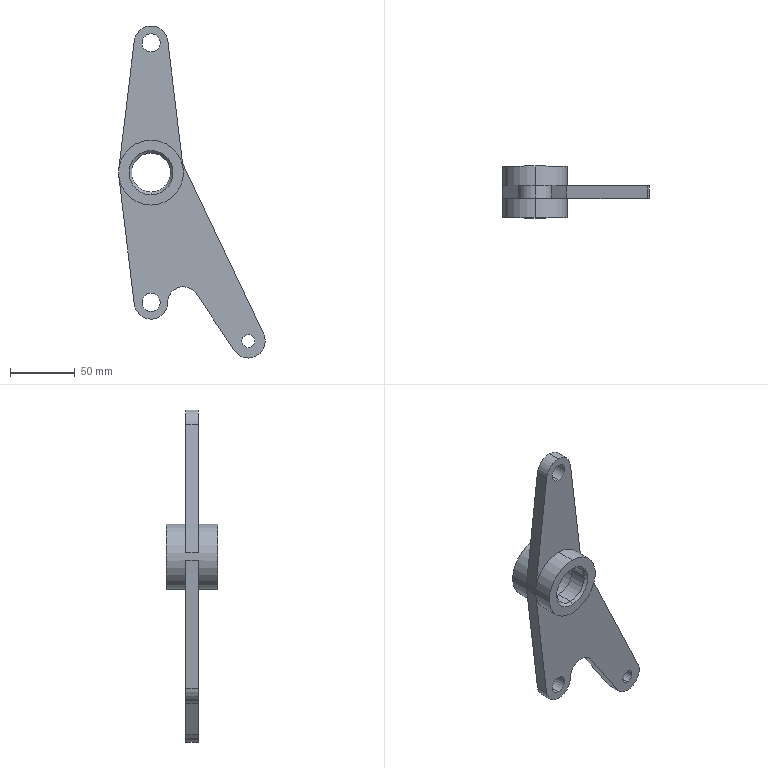Part | SolidWorks | features MirrorStock 1 | 1 solid | 37 faces | box 113 x 40 x 255.904 mm | volume 148805 mm3 | cylinder 21 | plane 12 | cone 4 | commonest cylinder face diameters 14 x4 26 x4 30 x4 50 x3 10 x2 24 x2
STEP:
#1=CARTESIAN_POINT('',(0.,-5.,-17.));
#2=VERTEX_POINT('',#1);
#3=CARTESIAN_POINT('',(0.,-5.,17.));
#4=VERTEX_POINT('',#3);
#5=CARTESIAN_POINT('',(0.,-5.,0.));
#6=DIRECTION('',(0.,-1.,0.));
#7=DIRECTION('',(0.,0.,-1.));
#8=AXIS2_PLACEMENT_3D('',#5,#6,#7);
#9=CIRCLE('',#8,17.);
#10=EDGE_CURVE('',#2,#4,#9,.T.);
#11=ORIENTED_EDGE('',*,*,#10,.T.);
#12=CARTESIAN_POINT('',(0.,5.,17.));
#13=VERTEX_POINT('',#12);
#14=CARTESIAN_POINT('',(0.,-5.,17.));
#15=DIRECTION('',(0.,1.,0.));
#16=VECTOR('',#15,1000.);
#17=LINE('',#14,#16);
#18=EDGE_CURVE('',#4,#13,#17,.T.);
#19=ORIENTED_EDGE('',*,*,#18,.T.);
#20=CARTESIAN_POINT('',(0.,5.,-17.));
#21=VERTEX_POINT('',#20);
#22=CARTESIAN_POINT('',(0.,5.,0.));
#23=DIRECTION('',(0.,-1.,0.));
#24=DIRECTION('',(0.,0.,-1.));
#25=AXIS2_PLACEMENT_3D('',#22,#23,#24);
#26=CIRCLE('',#25,17.);
#27=EDGE_CURVE('',#21,#13,#26,.T.);
#28=ORIENTED_EDGE('',*,*,#27,.F.);
#29=CARTESIAN_POINT('',(0.,-5.,-17.));
#30=DIRECTION('',(0.,1.,0.));
#31=VECTOR('',#30,1000.);
#32=LINE('',#29,#31);
#33=EDGE_CURVE('',#2,#21,#32,.T.);
#34=ORIENTED_EDGE('',*,*,#33,.F.);
#35=EDGE_LOOP('',(#11,#19,#28,#34));
#36=FACE_OUTER_BOUND('',#35,.T.);
#37=CARTESIAN_POINT('',(0.,-5.,0.));
#38=DIRECTION('',(0.,1.,0.));
#39=DIRECTION('',(0.,0.,-1.));
#40=AXIS2_PLACEMENT_3D('',#37,#38,#39);
#41=CYLINDRICAL_SURFACE('',#40,17.);
#42=ADVANCED_FACE('',(#36),#41,.F.);
#43=CARTESIAN_POINT('',(0.,18.,-15.));
#44=VERTEX_POINT('',#43);
#45=CARTESIAN_POINT('',(0.,18.,15.));
#46=VERTEX_POINT('',#45);
#47=CARTESIAN_POINT('',(0.,18.,0.));
#48=DIRECTION('',(0.,-1.,0.));
#49=DIRECTION('',(0.,0.,-1.));
#50=AXIS2_PLACEMENT_3D('',#47,#48,#49);
#51=CIRCLE('',#50,15.);
#52=EDGE_CURVE('',#44,#46,#51,.T.);
#53=ORIENTED_EDGE('',*,*,#52,.T.);
#54=CARTESIAN_POINT('',(0.,20.,17.));
#55=VERTEX_POINT('',#54);
#56=CARTESIAN_POINT('',(0.,18.,15.));
#57=DIRECTION('',(0.,0.7071,0.7071));
#58=VECTOR('',#57,1000.);
#59=LINE('',#56,#58);
#60=EDGE_CURVE('',#46,#55,#59,.T.);
#61=ORIENTED_EDGE('',*,*,#60,.T.);
#62=CARTESIAN_POINT('',(0.,20.,-17.));
#63=VERTEX_POINT('',#62);
#64=CARTESIAN_POINT('',(0.,20.,0.));
#65=DIRECTION('',(0.,1.,0.));
#66=DIRECTION('',(0.,0.,-1.));
#67=AXIS2_PLACEMENT_3D('',#64,#65,#66);
#68=CIRCLE('',#67,17.);
#69=EDGE_CURVE('',#55,#63,#68,.T.);
#70=ORIENTED_EDGE('',*,*,#69,.T.);
#71=CARTESIAN_POINT('',(0.,18.,-15.));
#72=DIRECTION('',(0.,0.7071,-0.7071));
#73=VECTOR('',#72,1000.);
#74=LINE('',#71,#73);
#75=EDGE_CURVE('',#44,#63,#74,.T.);
#76=ORIENTED_EDGE('',*,*,#75,.F.);
#77=EDGE_LOOP('',(#53,#61,#70,#76));
#78=FACE_OUTER_BOUND('',#77,.T.);
#79=CARTESIAN_POINT('',(0.,18.,0.));
#80=DIRECTION('',(0.,1.,0.));
#81=DIRECTION('',(0.,0.,-1.));
#82=AXIS2_PLACEMENT_3D('',#79,#80,#81);
#83=CONICAL_SURFACE('',#82,15.,0.7854);
#84=ADVANCED_FACE('',(#78),#83,.F.);
#85=CARTESIAN_POINT('',(0.,-18.,15.));
#86=VERTEX_POINT('',#85);
#87=CARTESIAN_POINT('',(0.,-18.,-15.));
#88=VERTEX_POINT('',#87);
#89=CARTESIAN_POINT('',(0.,-18.,0.));
#90=DIRECTION('',(0.,1.,0.));
#91=DIRECTION('',(0.,0.,-1.));
#92=AXIS2_PLACEMENT_3D('',#89,#90,#91);
#93=CIRCLE('',#92,15.);
#94=EDGE_CURVE('',#86,#88,#93,.T.);
#95=ORIENTED_EDGE('',*,*,#94,.T.);
#96=CARTESIAN_POINT('',(0.,-20.,-17.));
#97=VERTEX_POINT('',#96);
#98=CARTESIAN_POINT('',(0.,-20.,-17.));
#99=DIRECTION('',(0.,-0.7071,-0.7071));
#100=VECTOR('',#99,1000.);
#101=LINE('',#98,#100);
#102=EDGE_CURVE('',#88,#97,#101,.T.);
#103=ORIENTED_EDGE('',*,*,#102,.T.);
#104=CARTESIAN_POINT('',(0.,-20.,17.));
#105=VERTEX_POINT('',#104);
#106=CARTESIAN_POINT('',(0.,-20.,0.));
#107=DIRECTION('',(0.,-1.,0.));
#108=DIRECTION('',(0.,0.,-1.));
#109=AXIS2_PLACEMENT_3D('',#106,#107,#108);
#110=CIRCLE('',#109,17.);
#111=EDGE_CURVE('',#97,#105,#110,.T.);
#112=ORIENTED_EDGE('',*,*,#111,.T.);
#113=CARTESIAN_POINT('',(0.,-20.,17.));
#114=DIRECTION('',(0.,-0.7071,0.7071));
#115=VECTOR('',#114,1000.);
#116=LINE('',#113,#115);
#117=EDGE_CURVE('',#86,#105,#116,.T.);
#118=ORIENTED_EDGE('',*,*,#117,.F.);
#119=EDGE_LOOP('',(#95,#103,#112,#118));
#120=FACE_OUTER_BOUND('',#119,.T.);
#121=CARTESIAN_POINT('',(0.,-20.,0.));
#122=DIRECTION('',(0.,-1.,0.));
#123=DIRECTION('',(0.,0.,1.));
#124=AXIS2_PLACEMENT_3D('',#121,#122,#123);
#125=CONICAL_SURFACE('',#124,17.,0.7854);
#126=ADVANCED_FACE('',(#120),#125,.F.);
#127=CARTESIAN_POINT('',(75.,5.,-134.904));
#128=VERTEX_POINT('',#127);
#129=CARTESIAN_POINT('',(75.,5.,-124.904));
#130=VERTEX_POINT('',#129);
#131=CARTESIAN_POINT('',(75.,5.,-129.904));
#132=DIRECTION('',(0.,-1.,0.));
#133=DIRECTION('',(0.,0.,-1.));
#134=AXIS2_PLACEMENT_3D('',#131,#132,#133);
#135=CIRCLE('',#134,5.);
#136=EDGE_CURVE('',#128,#130,#135,.T.);
#137=ORIENTED_EDGE('',*,*,#136,.F.);
#138=CARTESIAN_POINT('',(75.,-5.,-134.904));
#139=VERTEX_POINT('',#138);
#140=CARTESIAN_POINT('',(75.,5.,-134.904));
#141=DIRECTION('',(0.,-1.,0.));
#142=VECTOR('',#141,1000.);
#143=LINE('',#140,#142);
#144=EDGE_CURVE('',#128,#139,#143,.T.);
#145=ORIENTED_EDGE('',*,*,#144,.T.);
#146=CARTESIAN_POINT('',(75.,-5.,-124.904));
#147=VERTEX_POINT('',#146);
#148=CARTESIAN_POINT('',(75.,-5.,-129.904));
#149=DIRECTION('',(0.,-1.,0.));
#150=DIRECTION('',(0.,0.,-1.));
#151=AXIS2_PLACEMENT_3D('',#148,#149,#150);
#152=CIRCLE('',#151,5.);
#153=EDGE_CURVE('',#139,#147,#152,.T.);
#154=ORIENTED_EDGE('',*,*,#153,.T.);
#155=CARTESIAN_POINT('',(75.,5.,-124.904));
#156=DIRECTION('',(0.,-1.,0.));
#157=VECTOR('',#156,1000.);
#158=LINE('',#155,#157);
#159=EDGE_CURVE('',#130,#147,#158,.T.);
#160=ORIENTED_EDGE('',*,*,#159,.F.);
#161=EDGE_LOOP('',(#137,#145,#154,#160));
#162=FACE_OUTER_BOUND('',#161,.T.);
#163=CARTESIAN_POINT('',(75.,5.,-129.904));
#164=DIRECTION('',(0.,-1.,0.));
#165=DIRECTION('',(0.,0.,1.));
#166=AXIS2_PLACEMENT_3D('',#163,#164,#165);
#167=CYLINDRICAL_SURFACE('',#166,5.);
#168=ADVANCED_FACE('',(#162),#167,.F.);
#169=CARTESIAN_POINT('',(0.,5.,-107.));
#170=VERTEX_POINT('',#169);
#171=CARTESIAN_POINT('',(0.,5.,-93.));
#172=VERTEX_POINT('',#171);
#173=CARTESIAN_POINT('',(0.,5.,-100.));
#174=DIRECTION('',(0.,-1.,0.));
#175=DIRECTION('',(0.,0.,1.));
#176=AXIS2_PLACEMENT_3D('',#173,#174,#175);
#177=CIRCLE('',#176,7.);
#178=EDGE_CURVE('',#170,#172,#177,.T.);
#179=ORIENTED_EDGE('',*,*,#178,.F.);
#180=CARTESIAN_POINT('',(0.,-5.,-107.));
#181=VERTEX_POINT('',#180);
#182=CARTESIAN_POINT('',(0.,5.,-107.));
#183=DIRECTION('',(0.,-1.,0.));
#184=VECTOR('',#183,1000.);
#185=LINE('',#182,#184);
#186=EDGE_CURVE('',#170,#181,#185,.T.);
#187=ORIENTED_EDGE('',*,*,#186,.T.);
#188=CARTESIAN_POINT('',(0.,-5.,-93.));
#189=VERTEX_POINT('',#188);
#190=CARTESIAN_POINT('',(0.,-5.,-100.));
#191=DIRECTION('',(0.,-1.,0.));
#192=DIRECTION('',(0.,0.,1.));
#193=AXIS2_PLACEMENT_3D('',#190,#191,#192);
#194=CIRCLE('',#193,7.);
#195=EDGE_CURVE('',#181,#189,#194,.T.);
#196=ORIENTED_EDGE('',*,*,#195,.T.);
#197=CARTESIAN_POINT('',(0.,5.,-93.));
#198=DIRECTION('',(0.,-1.,0.));
#199=VECTOR('',#198,1000.);
#200=LINE('',#197,#199);
#201=EDGE_CURVE('',#172,#189,#200,.T.);
#202=ORIENTED_EDGE('',*,*,#201,.F.);
#203=EDGE_LOOP('',(#179,#187,#196,#202));
#204=FACE_OUTER_BOUND('',#203,.T.);
#205=CARTESIAN_POINT('',(0.,5.,-100.));
#206=DIRECTION('',(0.,-1.,0.));
#207=DIRECTION('',(0.,0.,1.));
#208=AXIS2_PLACEMENT_3D('',#205,#206,#207);
#209=CYLINDRICAL_SURFACE('',#208,7.);
#210=ADVANCED_FACE('',(#204),#209,.F.);
#211=CARTESIAN_POINT('',(0.,5.,93.));
#212=VERTEX_POINT('',#211);
#213=CARTESIAN_POINT('',(0.,5.,107.));
#214=VERTEX_POINT('',#213);
#215=CARTESIAN_POINT('',(0.,5.,100.));
#216=DIRECTION('',(0.,-1.,0.));
#217=DIRECTION('',(0.,0.,-1.));
#218=AXIS2_PLACEMENT_3D('',#215,#216,#217);
#219=CIRCLE('',#218,7.);
#220=EDGE_CURVE('',#212,#214,#219,.T.);
#221=ORIENTED_EDGE('',*,*,#220,.F.);
#222=CARTESIAN_POINT('',(0.,-5.,93.));
#223=VERTEX_POINT('',#222);
#224=CARTESIAN_POINT('',(0.,5.,93.));
#225=DIRECTION('',(0.,-1.,0.));
#226=VECTOR('',#225,1000.);
#227=LINE('',#224,#226);
#228=EDGE_CURVE('',#212,#223,#227,.T.);
#229=ORIENTED_EDGE('',*,*,#228,.T.);
#230=CARTESIAN_POINT('',(0.,-5.,107.));
#231=VERTEX_POINT('',#230);
#232=CARTESIAN_POINT('',(0.,-5.,100.));
#233=DIRECTION('',(0.,-1.,0.));
#234=DIRECTION('',(0.,0.,-1.));
#235=AXIS2_PLACEMENT_3D('',#232,#233,#234);
#236=CIRCLE('',#235,7.);
#237=EDGE_CURVE('',#223,#231,#236,.T.);
#238=ORIENTED_EDGE('',*,*,#237,.T.);
#239=CARTESIAN_POINT('',(0.,5.,107.));
#240=DIRECTION('',(0.,-1.,0.));
#241=VECTOR('',#240,1000.);
#242=LINE('',#239,#241);
#243=EDGE_CURVE('',#214,#231,#242,.T.);
#244=ORIENTED_EDGE('',*,*,#243,.F.);
#245=EDGE_LOOP('',(#221,#229,#238,#244));
#246=FACE_OUTER_BOUND('',#245,.T.);
#247=CARTESIAN_POINT('',(0.,5.,100.));
#248=DIRECTION('',(0.,-1.,0.));
#249=DIRECTION('',(0.,0.,1.));
#250=AXIS2_PLACEMENT_3D('',#247,#248,#249);
#251=CYLINDRICAL_SURFACE('',#250,7.);
#252=ADVANCED_FACE('',(#246),#251,.F.);
#253=CARTESIAN_POINT('',(12.969,5.,-101.042));
#254=VERTEX_POINT('',#253);
#255=CARTESIAN_POINT('',(24.918,5.,-87.94));
#256=VERTEX_POINT('',#255);
#257=CARTESIAN_POINT('',(24.918,5.,-99.94));
#258=DIRECTION('',(0.,1.,0.));
#259=DIRECTION('',(0.,0.,-1.));
#260=AXIS2_PLACEMENT_3D('',#257,#258,#259);
#261=CIRCLE('',#260,12.);
#262=EDGE_CURVE('',#254,#256,#261,.T.);
#263=ORIENTED_EDGE('',*,*,#262,.T.);
#264=CARTESIAN_POINT('',(24.918,-5.,-87.94));
#265=VERTEX_POINT('',#264);
#266=CARTESIAN_POINT('',(24.918,5.,-87.94));
#267=DIRECTION('',(0.,-1.,0.));
#268=VECTOR('',#267,1000.);
#269=LINE('',#266,#268);
#270=EDGE_CURVE('',#256,#265,#269,.T.);
#271=ORIENTED_EDGE('',*,*,#270,.T.);
#272=CARTESIAN_POINT('',(12.969,-5.,-101.042));
#273=VERTEX_POINT('',#272);
#274=CARTESIAN_POINT('',(24.918,-5.,-99.94));
#275=DIRECTION('',(0.,1.,0.));
#276=DIRECTION('',(0.,0.,-1.));
#277=AXIS2_PLACEMENT_3D('',#274,#275,#276);
#278=CIRCLE('',#277,12.);
#279=EDGE_CURVE('',#273,#265,#278,.T.);
#280=ORIENTED_EDGE('',*,*,#279,.F.);
#281=CARTESIAN_POINT('',(12.969,5.,-101.042));
#282=DIRECTION('',(0.,-1.,0.));
#283=VECTOR('',#282,1000.);
#284=LINE('',#281,#283);
#285=EDGE_CURVE('',#254,#273,#284,.T.);
#286=ORIENTED_EDGE('',*,*,#285,.F.);
#287=EDGE_LOOP('',(#263,#271,#280,#286));
#288=FACE_OUTER_BOUND('',#287,.T.);
#289=CARTESIAN_POINT('',(24.918,5.,-99.94));
#290=DIRECTION('',(0.,-1.,0.));
#291=DIRECTION('',(0.,0.,1.));
#292=AXIS2_PLACEMENT_3D('',#289,#290,#291);
#293=CYLINDRICAL_SURFACE('',#292,12.);
#294=ADVANCED_FACE('',(#288),#293,.F.);
#295=CARTESIAN_POINT('',(12.906,5.,101.56));
#296=VERTEX_POINT('',#295);
#297=CARTESIAN_POINT('',(0.,5.,113.));
#298=VERTEX_POINT('',#297);
#299=CARTESIAN_POINT('',(0.,5.,100.));
#300=DIRECTION('',(0.,-1.,0.));
#301=DIRECTION('',(0.,0.,-1.));
#302=AXIS2_PLACEMENT_3D('',#299,#300,#301);
#303=CIRCLE('',#302,13.);
#304=EDGE_CURVE('',#296,#298,#303,.T.);
#305=ORIENTED_EDGE('',*,*,#304,.T.);
#306=CARTESIAN_POINT('',(0.,-5.,113.));
#307=VERTEX_POINT('',#306);
#308=CARTESIAN_POINT('',(0.,5.,113.));
#309=DIRECTION('',(0.,-1.,0.));
#310=VECTOR('',#309,1000.);
#311=LINE('',#308,#310);
#312=EDGE_CURVE('',#298,#307,#311,.T.);
#313=ORIENTED_EDGE('',*,*,#312,.T.);
#314=CARTESIAN_POINT('',(12.906,-5.,101.56));
#315=VERTEX_POINT('',#314);
#316=CARTESIAN_POINT('',(0.,-5.,100.));
#317=DIRECTION('',(0.,-1.,0.));
#318=DIRECTION('',(0.,0.,-1.));
#319=AXIS2_PLACEMENT_3D('',#316,#317,#318);
#320=CIRCLE('',#319,13.);
#321=EDGE_CURVE('',#315,#307,#320,.T.);
#322=ORIENTED_EDGE('',*,*,#321,.F.);
#323=CARTESIAN_POINT('',(12.906,5.,101.56));
#324=DIRECTION('',(0.,-1.,0.));
#325=VECTOR('',#324,1000.);
#326=LINE('',#323,#325);
#327=EDGE_CURVE('',#296,#315,#326,.T.);
#328=ORIENTED_EDGE('',*,*,#327,.F.);
#329=EDGE_LOOP('',(#305,#313,#322,#328));
#330=FACE_OUTER_BOUND('',#329,.T.);
#331=CARTESIAN_POINT('',(0.,5.,100.));
#332=DIRECTION('',(0.,-1.,0.));
#333=DIRECTION('',(0.,0.,1.));
#334=AXIS2_PLACEMENT_3D('',#331,#332,#333);
#335=CYLINDRICAL_SURFACE('',#334,13.);
#336=ADVANCED_FACE('',(#330),#335,.T.);
#337=ORIENTED_EDGE('',*,*,#52,.F.);
#338=CARTESIAN_POINT('',(0.,5.,-15.));
#339=VERTEX_POINT('',#338);
#340=CARTESIAN_POINT('',(0.,20.,-15.));
#341=DIRECTION('',(0.,-1.,0.));
#342=VECTOR('',#341,1000.);
#343=LINE('',#340,#342);
#344=EDGE_CURVE('',#44,#339,#343,.T.);
#345=ORIENTED_EDGE('',*,*,#344,.T.);
#346=CARTESIAN_POINT('',(0.,5.,15.));
#347=VERTEX_POINT('',#346);
#348=CARTESIAN_POINT('',(0.,5.,0.));
#349=DIRECTION('',(0.,-1.,0.));
#350=DIRECTION('',(0.,0.,-1.));
#351=AXIS2_PLACEMENT_3D('',#348,#349,#350);
#352=CIRCLE('',#351,15.);
#353=EDGE_CURVE('',#339,#347,#352,.T.);
#354=ORIENTED_EDGE('',*,*,#353,.T.);
#355=CARTESIAN_POINT('',(0.,20.,15.));
#356=DIRECTION('',(0.,-1.,0.));
#357=VECTOR('',#356,1000.);
#358=LINE('',#355,#357);
#359=EDGE_CURVE('',#46,#347,#358,.T.);
#360=ORIENTED_EDGE('',*,*,#359,.F.);
#361=EDGE_LOOP('',(#337,#345,#354,#360));
#362=FACE_OUTER_BOUND('',#361,.T.);
#363=CARTESIAN_POINT('',(0.,20.,0.));
#364=DIRECTION('',(0.,-1.,0.));
#365=DIRECTION('',(0.,0.,1.));
#366=AXIS2_PLACEMENT_3D('',#363,#364,#365);
#367=CYLINDRICAL_SURFACE('',#366,15.);
#368=ADVANCED_FACE('',(#362),#367,.F.);
#369=CARTESIAN_POINT('',(0.,20.,25.));
#370=VERTEX_POINT('',#369);
#371=CARTESIAN_POINT('',(0.,20.,-25.));
#372=VERTEX_POINT('',#371);
#373=CARTESIAN_POINT('',(0.,20.,0.));
#374=DIRECTION('',(0.,-1.,0.));
#375=DIRECTION('',(0.,0.,-1.));
#376=AXIS2_PLACEMENT_3D('',#373,#374,#375);
#377=CIRCLE('',#376,25.);
#378=EDGE_CURVE('',#370,#372,#377,.T.);
#379=ORIENTED_EDGE('',*,*,#378,.T.);
#380=CARTESIAN_POINT('',(0.,5.,-25.));
#381=VERTEX_POINT('',#380);
#382=CARTESIAN_POINT('',(0.,20.,-25.));
#383=DIRECTION('',(0.,-1.,0.));
#384=VECTOR('',#383,1000.);
#385=LINE('',#382,#384);
#386=EDGE_CURVE('',#372,#381,#385,.T.);
#387=ORIENTED_EDGE('',*,*,#386,.T.);
#388=CARTESIAN_POINT('',(-24.819,5.,-3.));
#389=VERTEX_POINT('',#388);
#390=CARTESIAN_POINT('',(0.,5.,0.));
#391=DIRECTION('',(0.,-1.,0.));
#392=DIRECTION('',(0.,0.,-1.));
#393=AXIS2_PLACEMENT_3D('',#390,#391,#392);
#394=CIRCLE('',#393,25.);
#395=EDGE_CURVE('',#389,#381,#394,.T.);
#396=ORIENTED_EDGE('',*,*,#395,.F.);
#397=CARTESIAN_POINT('',(-24.819,-5.,-3.));
#398=VERTEX_POINT('',#397);
#399=CARTESIAN_POINT('',(-24.819,5.,-3.));
#400=DIRECTION('',(0.,-1.,0.));
#401=VECTOR('',#400,1000.);
#402=LINE('',#399,#401);
#403=EDGE_CURVE('',#389,#398,#402,.T.);
#404=ORIENTED_EDGE('',*,*,#403,.T.);
#405=CARTESIAN_POINT('',(0.,-5.,-25.));
#406=VERTEX_POINT('',#405);
#407=CARTESIAN_POINT('',(0.,-5.,0.));
#408=DIRECTION('',(0.,-1.,0.));
#409=DIRECTION('',(0.,0.,-1.));
#410=AXIS2_PLACEMENT_3D('',#407,#408,#409);
#411=CIRCLE('',#410,25.);
#412=EDGE_CURVE('',#398,#406,#411,.T.);
#413=ORIENTED_EDGE('',*,*,#412,.T.);
#414=CARTESIAN_POINT('',(0.,-20.,-25.));
#415=VERTEX_POINT('',#414);
#416=CARTESIAN_POINT('',(0.,20.,-25.));
#417=DIRECTION('',(0.,-1.,0.));
#418=VECTOR('',#417,1000.);
#419=LINE('',#416,#418);
#420=EDGE_CURVE('',#406,#415,#419,.T.);
#421=ORIENTED_EDGE('',*,*,#420,.T.);
#422=CARTESIAN_POINT('',(0.,-20.,25.));
#423=VERTEX_POINT('',#422);
#424=CARTESIAN_POINT('',(0.,-20.,0.));
#425=DIRECTION('',(0.,-1.,0.));
#426=DIRECTION('',(0.,0.,-1.));
#427=AXIS2_PLACEMENT_3D('',#424,#425,#426);
#428=CIRCLE('',#427,25.);
#429=EDGE_CURVE('',#423,#415,#428,.T.);
#430=ORIENTED_EDGE('',*,*,#429,.F.);
#431=CARTESIAN_POINT('',(0.,-5.,25.));
#432=VERTEX_POINT('',#431);
#433=CARTESIAN_POINT('',(0.,20.,25.));
#434=DIRECTION('',(0.,-1.,0.));
#435=VECTOR('',#434,1000.);
#436=LINE('',#433,#435);
#437=EDGE_CURVE('',#432,#423,#436,.T.);
#438=ORIENTED_EDGE('',*,*,#437,.F.);
#439=CARTESIAN_POINT('',(-24.819,-5.,3.));
#440=VERTEX_POINT('',#439);
#441=CARTESIAN_POINT('',(0.,-5.,0.));
#442=DIRECTION('',(0.,-1.,0.));
#443=DIRECTION('',(0.,0.,-1.));
#444=AXIS2_PLACEMENT_3D('',#441,#442,#443);
#445=CIRCLE('',#444,25.);
#446=EDGE_CURVE('',#432,#440,#445,.T.);
#447=ORIENTED_EDGE('',*,*,#446,.T.);
#448=CARTESIAN_POINT('',(-24.819,5.,3.));
#449=VERTEX_POINT('',#448);
#450=CARTESIAN_POINT('',(-24.819,5.,3.));
#451=DIRECTION('',(0.,-1.,0.));
#452=VECTOR('',#451,1000.);
#453=LINE('',#450,#452);
#454=EDGE_CURVE('',#449,#440,#453,.T.);
#455=ORIENTED_EDGE('',*,*,#454,.F.);
#456=CARTESIAN_POINT('',(0.,5.,25.));
#457=VERTEX_POINT('',#456);
#458=CARTESIAN_POINT('',(0.,5.,0.));
#459=DIRECTION('',(0.,-1.,0.));
#460=DIRECTION('',(0.,0.,-1.));
#461=AXIS2_PLACEMENT_3D('',#458,#459,#460);
#462=CIRCLE('',#461,25.);
#463=EDGE_CURVE('',#457,#449,#462,.T.);
#464=ORIENTED_EDGE('',*,*,#463,.F.);
#465=CARTESIAN_POINT('',(0.,20.,25.));
#466=DIRECTION('',(0.,-1.,0.));
#467=VECTOR('',#466,1000.);
#468=LINE('',#465,#467);
#469=EDGE_CURVE('',#370,#457,#468,.T.);
#470=ORIENTED_EDGE('',*,*,#469,.F.);
#471=EDGE_LOOP('',(#379,#387,#396,#404,#413,#421,#430,#438,#447,#455,#464,#470));
#472=FACE_OUTER_BOUND('',#471,.T.);
#473=CARTESIAN_POINT('',(0.,20.,0.));
#474=DIRECTION('',(0.,-1.,0.));
#475=DIRECTION('',(0.,0.,1.));
#476=AXIS2_PLACEMENT_3D('',#473,#474,#475);
#477=CYLINDRICAL_SURFACE('',#476,25.);
#478=ADVANCED_FACE('',(#472),#477,.T.);
#479=ORIENTED_EDGE('',*,*,#386,.F.);
#480=CARTESIAN_POINT('',(0.,20.,0.));
#481=DIRECTION('',(0.,-1.,0.));
#482=DIRECTION('',(0.,0.,-1.));
#483=AXIS2_PLACEMENT_3D('',#480,#481,#482);
#484=CIRCLE('',#483,25.);
#485=EDGE_CURVE('',#372,#370,#484,.T.);
#486=ORIENTED_EDGE('',*,*,#485,.T.);
#487=ORIENTED_EDGE('',*,*,#469,.T.);
#488=CARTESIAN_POINT('',(0.,5.,0.));
#489=DIRECTION('',(0.,-1.,0.));
#490=DIRECTION('',(0.,0.,-1.));
#491=AXIS2_PLACEMENT_3D('',#488,#489,#490);
#492=CIRCLE('',#491,25.);
#493=EDGE_CURVE('',#381,#457,#492,.T.);
#494=ORIENTED_EDGE('',*,*,#493,.F.);
#495=EDGE_LOOP('',(#479,#486,#487,#494));
#496=FACE_OUTER_BOUND('',#495,.T.);
#497=CARTESIAN_POINT('',(0.,20.,0.));
#498=DIRECTION('',(0.,-1.,0.));
#499=DIRECTION('',(0.,0.,1.));
#500=AXIS2_PLACEMENT_3D('',#497,#498,#499);
#501=CYLINDRICAL_SURFACE('',#500,25.);
#502=ADVANCED_FACE('',(#496),#501,.T.);
#503=CARTESIAN_POINT('',(0.,-5.,-15.));
#504=VERTEX_POINT('',#503);
#505=CARTESIAN_POINT('',(0.,-5.,15.));
#506=VERTEX_POINT('',#505);
#507=CARTESIAN_POINT('',(0.,-5.,0.));
#508=DIRECTION('',(0.,-1.,0.));
#509=DIRECTION('',(0.,0.,-1.));
#510=AXIS2_PLACEMENT_3D('',#507,#508,#509);
#511=CIRCLE('',#510,15.);
#512=EDGE_CURVE('',#504,#506,#511,.T.);
#513=ORIENTED_EDGE('',*,*,#512,.F.);
#514=CARTESIAN_POINT('',(0.,20.,-15.));
#515=DIRECTION('',(0.,-1.,0.));
#516=VECTOR('',#515,1000.);
#517=LINE('',#514,#516);
#518=EDGE_CURVE('',#504,#88,#517,.T.);
#519=ORIENTED_EDGE('',*,*,#518,.T.);
#520=ORIENTED_EDGE('',*,*,#94,.F.);
#521=CARTESIAN_POINT('',(0.,20.,15.));
#522=DIRECTION('',(0.,-1.,0.));
#523=VECTOR('',#522,1000.);
#524=LINE('',#521,#523);
#525=EDGE_CURVE('',#506,#86,#524,.T.);
#526=ORIENTED_EDGE('',*,*,#525,.F.);
#527=EDGE_LOOP('',(#513,#519,#520,#526));
#528=FACE_OUTER_BOUND('',#527,.T.);
#529=CARTESIAN_POINT('',(0.,20.,0.));
#530=DIRECTION('',(0.,-1.,0.));
#531=DIRECTION('',(0.,0.,1.));
#532=AXIS2_PLACEMENT_3D('',#529,#530,#531);
#533=CYLINDRICAL_SURFACE('',#532,15.);
#534=ADVANCED_FACE('',(#528),#533,.F.);
#535=ORIENTED_EDGE('',*,*,#518,.F.);
#536=CARTESIAN_POINT('',(0.,-5.,0.));
#537=DIRECTION('',(0.,-1.,0.));
#538=DIRECTION('',(0.,0.,-1.));
#539=AXIS2_PLACEMENT_3D('',#536,#537,#538);
#540=CIRCLE('',#539,15.);
#541=EDGE_CURVE('',#506,#504,#540,.T.);
#542=ORIENTED_EDGE('',*,*,#541,.F.);
#543=ORIENTED_EDGE('',*,*,#525,.T.);
#544=CARTESIAN_POINT('',(0.,-18.,0.));
#545=DIRECTION('',(0.,1.,0.));
#546=DIRECTION('',(0.,0.,-1.));
#547=AXIS2_PLACEMENT_3D('',#544,#545,#546);
#548=CIRCLE('',#547,15.);
#549=EDGE_CURVE('',#88,#86,#548,.T.);
#550=ORIENTED_EDGE('',*,*,#549,.F.);
#551=EDGE_LOOP('',(#535,#542,#543,#550));
#552=FACE_OUTER_BOUND('',#551,.T.);
#553=CARTESIAN_POINT('',(0.,20.,0.));
#554=DIRECTION('',(0.,-1.,0.));
#555=DIRECTION('',(0.,0.,1.));
#556=AXIS2_PLACEMENT_3D('',#553,#554,#555);
#557=CYLINDRICAL_SURFACE('',#556,15.);
#558=ADVANCED_FACE('',(#552),#557,.F.);
#559=CARTESIAN_POINT('',(0.,20.,0.));
#560=DIRECTION('',(0.,1.,0.));
#561=DIRECTION('',(0.,0.,-1.));
#562=AXIS2_PLACEMENT_3D('',#559,#560,#561);
#563=CIRCLE('',#562,17.);
#564=EDGE_CURVE('',#63,#55,#563,.T.);
#565=ORIENTED_EDGE('',*,*,#564,.F.);
#566=ORIENTED_EDGE('',*,*,#69,.F.);
#567=EDGE_LOOP('',(#565,#566));
#568=FACE_BOUND('',#567,.T.);
#569=ORIENTED_EDGE('',*,*,#378,.F.);
#570=ORIENTED_EDGE('',*,*,#485,.F.);
#571=EDGE_LOOP('',(#569,#570));
#572=FACE_OUTER_BOUND('',#571,.T.);
#573=CARTESIAN_POINT('',(0.,20.,0.));
#574=DIRECTION('',(0.,1.,0.));
#575=DIRECTION('',(0.,0.,-1.));
#576=AXIS2_PLACEMENT_3D('',#573,#574,#575);
#577=PLANE('',#576);
#578=ADVANCED_FACE('',(#568,#572),#577,.T.);
#579=CARTESIAN_POINT('',(0.,-20.,0.));
#580=DIRECTION('',(0.,-1.,0.));
#581=DIRECTION('',(0.,0.,-1.));
#582=AXIS2_PLACEMENT_3D('',#579,#580,#581);
#583=CIRCLE('',#582,17.);
#584=EDGE_CURVE('',#105,#97,#583,.T.);
#585=ORIENTED_EDGE('',*,*,#584,.F.);
#586=ORIENTED_EDGE('',*,*,#111,.F.);
#587=EDGE_LOOP('',(#585,#586));
#588=FACE_BOUND('',#587,.T.);
#589=ORIENTED_EDGE('',*,*,#429,.T.);
#590=CARTESIAN_POINT('',(0.,-20.,0.));
#591=DIRECTION('',(0.,-1.,0.));
#592=DIRECTION('',(0.,0.,-1.));
#593=AXIS2_PLACEMENT_3D('',#590,#591,#592);
#594=CIRCLE('',#593,25.);
#595=EDGE_CURVE('',#415,#423,#594,.T.);
#596=ORIENTED_EDGE('',*,*,#595,.T.);
#597=EDGE_LOOP('',(#589,#596));
#598=FACE_OUTER_BOUND('',#597,.T.);
#599=CARTESIAN_POINT('',(0.,-20.,0.));
#600=DIRECTION('',(0.,1.,0.));
#601=DIRECTION('',(0.,0.,-1.));
#602=AXIS2_PLACEMENT_3D('',#599,#600,#601);
#603=PLANE('',#602);
#604=ADVANCED_FACE('',(#588,#598),#603,.F.);
#605=ORIENTED_EDGE('',*,*,#420,.F.);
#606=CARTESIAN_POINT('',(0.,-5.,0.));
#607=DIRECTION('',(0.,-1.,0.));
#608=DIRECTION('',(0.,0.,-1.));
#609=AXIS2_PLACEMENT_3D('',#606,#607,#608);
#610=CIRCLE('',#609,25.);
#611=EDGE_CURVE('',#406,#432,#610,.T.);
#612=ORIENTED_EDGE('',*,*,#611,.T.);
#613=ORIENTED_EDGE('',*,*,#437,.T.);
#614=ORIENTED_EDGE('',*,*,#595,.F.);
#615=EDGE_LOOP('',(#605,#612,#613,#614));
#616=FACE_OUTER_BOUND('',#615,.T.);
#617=CARTESIAN_POINT('',(0.,20.,0.));
#618=DIRECTION('',(0.,-1.,0.));
#619=DIRECTION('',(0.,0.,1.));
#620=AXIS2_PLACEMENT_3D('',#617,#618,#619);
#621=CYLINDRICAL_SURFACE('',#620,25.);
#622=ADVANCED_FACE('',(#616),#621,.T.);
#623=ORIENTED_EDGE('',*,*,#344,.F.);
#624=CARTESIAN_POINT('',(0.,18.,0.));
#625=DIRECTION('',(0.,-1.,0.));
#626=DIRECTION('',(0.,0.,-1.));
#627=AXIS2_PLACEMENT_3D('',#624,#625,#626);
#628=CIRCLE('',#627,15.);
#629=EDGE_CURVE('',#46,#44,#628,.T.);
#630=ORIENTED_EDGE('',*,*,#629,.F.);
#631=ORIENTED_EDGE('',*,*,#359,.T.);
#632=CARTESIAN_POINT('',(0.,5.,0.));
#633=DIRECTION('',(0.,-1.,0.));
#634=DIRECTION('',(0.,0.,-1.));
#635=AXIS2_PLACEMENT_3D('',#632,#633,#634);
#636=CIRCLE('',#635,15.);
#637=EDGE_CURVE('',#347,#339,#636,.T.);
#638=ORIENTED_EDGE('',*,*,#637,.T.);
#639=EDGE_LOOP('',(#623,#630,#631,#638));
#640=FACE_OUTER_BOUND('',#639,.T.);
#641=CARTESIAN_POINT('',(0.,20.,0.));
#642=DIRECTION('',(0.,-1.,0.));
#643=DIRECTION('',(0.,0.,1.));
#644=AXIS2_PLACEMENT_3D('',#641,#642,#643);
#645=CYLINDRICAL_SURFACE('',#644,15.);
#646=ADVANCED_FACE('',(#640),#645,.F.);
#647=CARTESIAN_POINT('',(75.,5.,-129.904));
#648=DIRECTION('',(0.,-1.,0.));
#649=DIRECTION('',(0.,0.,-1.));
#650=AXIS2_PLACEMENT_3D('',#647,#648,#649);
#651=CIRCLE('',#650,5.);
#652=EDGE_CURVE('',#130,#128,#651,.T.);
#653=ORIENTED_EDGE('',*,*,#652,.T.);
#654=ORIENTED_EDGE('',*,*,#136,.T.);
#655=EDGE_LOOP('',(#653,#654));
#656=FACE_BOUND('',#655,.T.);
#657=CARTESIAN_POINT('',(0.,5.,100.));
#658=DIRECTION('',(0.,-1.,0.));
#659=DIRECTION('',(0.,0.,-1.));
#660=AXIS2_PLACEMENT_3D('',#657,#658,#659);
#661=CIRCLE('',#660,7.);
#662=EDGE_CURVE('',#214,#212,#661,.T.);
#663=ORIENTED_EDGE('',*,*,#662,.T.);
#664=ORIENTED_EDGE('',*,*,#220,.T.);
#665=EDGE_LOOP('',(#663,#664));
#666=FACE_BOUND('',#665,.T.);
#667=CARTESIAN_POINT('',(0.,5.,-100.));
#668=DIRECTION('',(0.,-1.,0.));
#669=DIRECTION('',(0.,0.,1.));
#670=AXIS2_PLACEMENT_3D('',#667,#668,#669);
#671=CIRCLE('',#670,7.);
#672=EDGE_CURVE('',#172,#170,#671,.T.);
#673=ORIENTED_EDGE('',*,*,#672,.T.);
#674=ORIENTED_EDGE('',*,*,#178,.T.);
#675=EDGE_LOOP('',(#673,#674));
#676=FACE_BOUND('',#675,.T.);
#677=ORIENTED_EDGE('',*,*,#395,.T.);
#678=ORIENTED_EDGE('',*,*,#493,.T.);
#679=ORIENTED_EDGE('',*,*,#463,.T.);
#680=CARTESIAN_POINT('',(-12.906,5.,101.56));
#681=VERTEX_POINT('',#680);
#682=CARTESIAN_POINT('',(-12.906,5.,101.56));
#683=DIRECTION('',(-0.12,0.,-0.9928));
#684=VECTOR('',#683,1000.);
#685=LINE('',#682,#684);
#686=EDGE_CURVE('',#681,#449,#685,.T.);
#687=ORIENTED_EDGE('',*,*,#686,.F.);
#688=CARTESIAN_POINT('',(0.,5.,100.));
#689=DIRECTION('',(0.,-1.,0.));
#690=DIRECTION('',(0.,0.,-1.));
#691=AXIS2_PLACEMENT_3D('',#688,#689,#690);
#692=CIRCLE('',#691,13.);
#693=EDGE_CURVE('',#298,#681,#692,.T.);
#694=ORIENTED_EDGE('',*,*,#693,.F.);
#695=ORIENTED_EDGE('',*,*,#304,.F.);
#696=CARTESIAN_POINT('',(24.33,5.,7.046));
#697=VERTEX_POINT('',#696);
#698=CARTESIAN_POINT('',(12.906,5.,101.56));
#699=DIRECTION('',(-0.12,0.,0.9928));
#700=VECTOR('',#699,1000.);
#701=LINE('',#698,#700);
#702=EDGE_CURVE('',#697,#296,#701,.T.);
#703=ORIENTED_EDGE('',*,*,#702,.F.);
#704=CARTESIAN_POINT('',(86.742,5.,-124.325));
#705=VERTEX_POINT('',#704);
#706=CARTESIAN_POINT('',(24.33,5.,7.046));
#707=DIRECTION('',(-0.4291,0.,0.9032));
#708=VECTOR('',#707,1000.);
#709=LINE('',#706,#708);
#710=EDGE_CURVE('',#705,#697,#709,.T.);
#711=ORIENTED_EDGE('',*,*,#710,.F.);
#712=CARTESIAN_POINT('',(64.19,5.,-137.125));
#713=VERTEX_POINT('',#712);
#714=CARTESIAN_POINT('',(75.,5.,-129.904));
#715=DIRECTION('',(0.,-1.,0.));
#716=DIRECTION('',(0.,0.,-1.));
#717=AXIS2_PLACEMENT_3D('',#714,#715,#716);
#718=CIRCLE('',#717,13.);
#719=EDGE_CURVE('',#713,#705,#718,.T.);
#720=ORIENTED_EDGE('',*,*,#719,.F.);
#721=CARTESIAN_POINT('',(34.896,5.,-93.275));
#722=VERTEX_POINT('',#721);
#723=CARTESIAN_POINT('',(64.19,5.,-137.125));
#724=DIRECTION('',(0.5555,0.,-0.8315));
#725=VECTOR('',#724,1000.);
#726=LINE('',#723,#725);
#727=EDGE_CURVE('',#722,#713,#726,.T.);
#728=ORIENTED_EDGE('',*,*,#727,.F.);
#729=CARTESIAN_POINT('',(24.918,5.,-99.94));
#730=DIRECTION('',(0.,1.,0.));
#731=DIRECTION('',(0.,0.,-1.));
#732=AXIS2_PLACEMENT_3D('',#729,#730,#731);
#733=CIRCLE('',#732,12.);
#734=EDGE_CURVE('',#256,#722,#733,.T.);
#735=ORIENTED_EDGE('',*,*,#734,.F.);
#736=ORIENTED_EDGE('',*,*,#262,.F.);
#737=CARTESIAN_POINT('',(12.906,5.,-101.56));
#738=VERTEX_POINT('',#737);
#739=CARTESIAN_POINT('',(12.906,5.,-101.56));
#740=DIRECTION('',(0.12,0.,0.9928));
#741=VECTOR('',#740,1000.);
#742=LINE('',#739,#741);
#743=EDGE_CURVE('',#738,#254,#742,.T.);
#744=ORIENTED_EDGE('',*,*,#743,.F.);
#745=CARTESIAN_POINT('',(-12.906,5.,-101.56));
#746=VERTEX_POINT('',#745);
#747=CARTESIAN_POINT('',(0.,5.,-100.));
#748=DIRECTION('',(0.,-1.,0.));
#749=DIRECTION('',(0.,0.,1.));
#750=AXIS2_PLACEMENT_3D('',#747,#748,#749);
#751=CIRCLE('',#750,13.);
#752=EDGE_CURVE('',#746,#738,#751,.T.);
#753=ORIENTED_EDGE('',*,*,#752,.F.);
#754=CARTESIAN_POINT('',(-12.906,5.,-101.56));
#755=DIRECTION('',(0.12,0.,-0.9928));
#756=VECTOR('',#755,1000.);
#757=LINE('',#754,#756);
#758=EDGE_CURVE('',#389,#746,#757,.T.);
#759=ORIENTED_EDGE('',*,*,#758,.F.);
#760=EDGE_LOOP('',(#677,#678,#679,#687,#694,#695,#703,#711,#720,#728,#735,#736,#744,#753,#759));
#761=FACE_OUTER_BOUND('',#760,.T.);
#762=CARTESIAN_POINT('',(75.,5.,-129.904));
#763=DIRECTION('',(0.,1.,0.));
#764=DIRECTION('',(0.,0.,-1.));
#765=AXIS2_PLACEMENT_3D('',#762,#763,#764);
#766=PLANE('',#765);
#767=ADVANCED_FACE('',(#656,#666,#676,#761),#766,.T.);
#768=CARTESIAN_POINT('',(75.,-5.,-129.904));
#769=DIRECTION('',(0.,-1.,0.));
#770=DIRECTION('',(0.,0.,-1.));
#771=AXIS2_PLACEMENT_3D('',#768,#769,#770);
#772=CIRCLE('',#771,5.);
#773=EDGE_CURVE('',#147,#139,#772,.T.);
#774=ORIENTED_EDGE('',*,*,#773,.F.);
#775=ORIENTED_EDGE('',*,*,#153,.F.);
#776=EDGE_LOOP('',(#774,#775));
#777=FACE_BOUND('',#776,.T.);
#778=CARTESIAN_POINT('',(0.,-5.,-100.));
#779=DIRECTION('',(0.,-1.,0.));
#780=DIRECTION('',(0.,0.,1.));
#781=AXIS2_PLACEMENT_3D('',#778,#779,#780);
#782=CIRCLE('',#781,7.);
#783=EDGE_CURVE('',#189,#181,#782,.T.);
#784=ORIENTED_EDGE('',*,*,#783,.F.);
#785=ORIENTED_EDGE('',*,*,#195,.F.);
#786=EDGE_LOOP('',(#784,#785));
#787=FACE_BOUND('',#786,.T.);
#788=CARTESIAN_POINT('',(0.,-5.,100.));
#789=DIRECTION('',(0.,-1.,0.));
#790=DIRECTION('',(0.,0.,-1.));
#791=AXIS2_PLACEMENT_3D('',#788,#789,#790);
#792=CIRCLE('',#791,7.);
#793=EDGE_CURVE('',#231,#223,#792,.T.);
#794=ORIENTED_EDGE('',*,*,#793,.F.);
#795=ORIENTED_EDGE('',*,*,#237,.F.);
#796=EDGE_LOOP('',(#794,#795));
#797=FACE_BOUND('',#796,.T.);
#798=CARTESIAN_POINT('',(-12.906,-5.,-101.56));
#799=VERTEX_POINT('',#798);
#800=CARTESIAN_POINT('',(-12.906,-5.,-101.56));
#801=DIRECTION('',(0.12,0.,-0.9928));
#802=VECTOR('',#801,1000.);
#803=LINE('',#800,#802);
#804=EDGE_CURVE('',#398,#799,#803,.T.);
#805=ORIENTED_EDGE('',*,*,#804,.T.);
#806=CARTESIAN_POINT('',(12.906,-5.,-101.56));
#807=VERTEX_POINT('',#806);
#808=CARTESIAN_POINT('',(0.,-5.,-100.));
#809=DIRECTION('',(0.,-1.,0.));
#810=DIRECTION('',(0.,0.,1.));
#811=AXIS2_PLACEMENT_3D('',#808,#809,#810);
#812=CIRCLE('',#811,13.);
#813=EDGE_CURVE('',#799,#807,#812,.T.);
#814=ORIENTED_EDGE('',*,*,#813,.T.);
#815=CARTESIAN_POINT('',(12.906,-5.,-101.56));
#816=DIRECTION('',(0.12,0.,0.9928));
#817=VECTOR('',#816,1000.);
#818=LINE('',#815,#817);
#819=EDGE_CURVE('',#807,#273,#818,.T.);
#820=ORIENTED_EDGE('',*,*,#819,.T.);
#821=ORIENTED_EDGE('',*,*,#279,.T.);
#822=CARTESIAN_POINT('',(34.896,-5.,-93.275));
#823=VERTEX_POINT('',#822);
#824=CARTESIAN_POINT('',(24.918,-5.,-99.94));
#825=DIRECTION('',(0.,1.,0.));
#826=DIRECTION('',(0.,0.,-1.));
#827=AXIS2_PLACEMENT_3D('',#824,#825,#826);
#828=CIRCLE('',#827,12.);
#829=EDGE_CURVE('',#265,#823,#828,.T.);
#830=ORIENTED_EDGE('',*,*,#829,.T.);
#831=CARTESIAN_POINT('',(64.19,-5.,-137.125));
#832=VERTEX_POINT('',#831);
#833=CARTESIAN_POINT('',(64.19,-5.,-137.125));
#834=DIRECTION('',(0.5555,0.,-0.8315));
#835=VECTOR('',#834,1000.);
#836=LINE('',#833,#835);
#837=EDGE_CURVE('',#823,#832,#836,.T.);
#838=ORIENTED_EDGE('',*,*,#837,.T.);
#839=CARTESIAN_POINT('',(86.742,-5.,-124.325));
#840=VERTEX_POINT('',#839);
#841=CARTESIAN_POINT('',(75.,-5.,-129.904));
#842=DIRECTION('',(0.,-1.,0.));
#843=DIRECTION('',(0.,0.,-1.));
#844=AXIS2_PLACEMENT_3D('',#841,#842,#843);
#845=CIRCLE('',#844,13.);
#846=EDGE_CURVE('',#832,#840,#845,.T.);
#847=ORIENTED_EDGE('',*,*,#846,.T.);
#848=CARTESIAN_POINT('',(24.33,-5.,7.046));
#849=VERTEX_POINT('',#848);
#850=CARTESIAN_POINT('',(24.33,-5.,7.046));
#851=DIRECTION('',(-0.4291,0.,0.9032));
#852=VECTOR('',#851,1000.);
#853=LINE('',#850,#852);
#854=EDGE_CURVE('',#840,#849,#853,.T.);
#855=ORIENTED_EDGE('',*,*,#854,.T.);
#856=CARTESIAN_POINT('',(12.906,-5.,101.56));
#857=DIRECTION('',(-0.12,0.,0.9928));
#858=VECTOR('',#857,1000.);
#859=LINE('',#856,#858);
#860=EDGE_CURVE('',#849,#315,#859,.T.);
#861=ORIENTED_EDGE('',*,*,#860,.T.);
#862=ORIENTED_EDGE('',*,*,#321,.T.);
#863=CARTESIAN_POINT('',(-12.906,-5.,101.56));
#864=VERTEX_POINT('',#863);
#865=CARTESIAN_POINT('',(0.,-5.,100.));
#866=DIRECTION('',(0.,-1.,0.));
#867=DIRECTION('',(0.,0.,-1.));
#868=AXIS2_PLACEMENT_3D('',#865,#866,#867);
#869=CIRCLE('',#868,13.);
#870=EDGE_CURVE('',#307,#864,#869,.T.);
#871=ORIENTED_EDGE('',*,*,#870,.T.);
#872=CARTESIAN_POINT('',(-12.906,-5.,101.56));
#873=DIRECTION('',(-0.12,0.,-0.9928));
#874=VECTOR('',#873,1000.);
#875=LINE('',#872,#874);
#876=EDGE_CURVE('',#864,#440,#875,.T.);
#877=ORIENTED_EDGE('',*,*,#876,.T.);
#878=ORIENTED_EDGE('',*,*,#446,.F.);
#879=ORIENTED_EDGE('',*,*,#611,.F.);
#880=ORIENTED_EDGE('',*,*,#412,.F.);
#881=EDGE_LOOP('',(#805,#814,#820,#821,#830,#838,#847,#855,#861,#862,#871,#877,#878,#879,#880));
#882=FACE_OUTER_BOUND('',#881,.T.);
#883=CARTESIAN_POINT('',(75.,-5.,-129.904));
#884=DIRECTION('',(0.,1.,0.));
#885=DIRECTION('',(0.,0.,-1.));
#886=AXIS2_PLACEMENT_3D('',#883,#884,#885);
#887=PLANE('',#886);
#888=ADVANCED_FACE('',(#777,#787,#797,#882),#887,.F.);
#889=ORIENTED_EDGE('',*,*,#846,.F.);
#890=CARTESIAN_POINT('',(64.19,5.,-137.125));
#891=DIRECTION('',(0.,-1.,0.));
#892=VECTOR('',#891,1000.);
#893=LINE('',#890,#892);
#894=EDGE_CURVE('',#713,#832,#893,.T.);
#895=ORIENTED_EDGE('',*,*,#894,.F.);
#896=ORIENTED_EDGE('',*,*,#719,.T.);
#897=CARTESIAN_POINT('',(86.742,5.,-124.325));
#898=DIRECTION('',(0.,-1.,0.));
#899=VECTOR('',#898,1000.);
#900=LINE('',#897,#899);
#901=EDGE_CURVE('',#705,#840,#900,.T.);
#902=ORIENTED_EDGE('',*,*,#901,.T.);
#903=EDGE_LOOP('',(#889,#895,#896,#902));
#904=FACE_OUTER_BOUND('',#903,.T.);
#905=CARTESIAN_POINT('',(75.,5.,-129.904));
#906=DIRECTION('',(0.,-1.,0.));
#907=DIRECTION('',(0.,0.,1.));
#908=AXIS2_PLACEMENT_3D('',#905,#906,#907);
#909=CYLINDRICAL_SURFACE('',#908,13.);
#910=ADVANCED_FACE('',(#904),#909,.T.);
#911=ORIENTED_EDGE('',*,*,#854,.F.);
#912=ORIENTED_EDGE('',*,*,#901,.F.);
#913=ORIENTED_EDGE('',*,*,#710,.T.);
#914=CARTESIAN_POINT('',(24.33,5.,7.046));
#915=DIRECTION('',(0.,-1.,0.));
#916=VECTOR('',#915,1000.);
#917=LINE('',#914,#916);
#918=EDGE_CURVE('',#697,#849,#917,.T.);
#919=ORIENTED_EDGE('',*,*,#918,.T.);
#920=EDGE_LOOP('',(#911,#912,#913,#919));
#921=FACE_OUTER_BOUND('',#920,.T.);
#922=CARTESIAN_POINT('',(24.33,5.,7.046));
#923=DIRECTION('',(-0.9032,0.,-0.4291));
#924=DIRECTION('',(0.4291,0.,-0.9032));
#925=AXIS2_PLACEMENT_3D('',#922,#923,#924);
#926=PLANE('',#925);
#927=ADVANCED_FACE('',(#921),#926,.F.);
#928=ORIENTED_EDGE('',*,*,#860,.F.);
#929=ORIENTED_EDGE('',*,*,#918,.F.);
#930=ORIENTED_EDGE('',*,*,#702,.T.);
#931=ORIENTED_EDGE('',*,*,#327,.T.);
#932=EDGE_LOOP('',(#928,#929,#930,#931));
#933=FACE_OUTER_BOUND('',#932,.T.);
#934=CARTESIAN_POINT('',(12.906,5.,101.56));
#935=DIRECTION('',(-0.9928,0.,-0.12));
#936=DIRECTION('',(0.12,0.,-0.9928));
#937=AXIS2_PLACEMENT_3D('',#934,#935,#936);
#938=PLANE('',#937);
#939=ADVANCED_FACE('',(#933),#938,.F.);
#940=ORIENTED_EDGE('',*,*,#312,.F.);
#941=ORIENTED_EDGE('',*,*,#693,.T.);
#942=CARTESIAN_POINT('',(-12.906,5.,101.56));
#943=DIRECTION('',(0.,-1.,0.));
#944=VECTOR('',#943,1000.);
#945=LINE('',#942,#944);
#946=EDGE_CURVE('',#681,#864,#945,.T.);
#947=ORIENTED_EDGE('',*,*,#946,.T.);
#948=ORIENTED_EDGE('',*,*,#870,.F.);
#949=EDGE_LOOP('',(#940,#941,#947,#948));
#950=FACE_OUTER_BOUND('',#949,.T.);
#951=CARTESIAN_POINT('',(0.,5.,100.));
#952=DIRECTION('',(0.,-1.,0.));
#953=DIRECTION('',(0.,0.,1.));
#954=AXIS2_PLACEMENT_3D('',#951,#952,#953);
#955=CYLINDRICAL_SURFACE('',#954,13.);
#956=ADVANCED_FACE('',(#950),#955,.T.);
#957=ORIENTED_EDGE('',*,*,#876,.F.);
#958=ORIENTED_EDGE('',*,*,#946,.F.);
#959=ORIENTED_EDGE('',*,*,#686,.T.);
#960=ORIENTED_EDGE('',*,*,#454,.T.);
#961=EDGE_LOOP('',(#957,#958,#959,#960));
#962=FACE_OUTER_BOUND('',#961,.T.);
#963=CARTESIAN_POINT('',(-12.906,5.,101.56));
#964=DIRECTION('',(0.9928,0.,-0.12));
#965=DIRECTION('',(0.12,0.,0.9928));
#966=AXIS2_PLACEMENT_3D('',#963,#964,#965);
#967=PLANE('',#966);
#968=ADVANCED_FACE('',(#962),#967,.F.);
#969=ORIENTED_EDGE('',*,*,#804,.F.);
#970=ORIENTED_EDGE('',*,*,#403,.F.);
#971=ORIENTED_EDGE('',*,*,#758,.T.);
#972=CARTESIAN_POINT('',(-12.906,5.,-101.56));
#973=DIRECTION('',(0.,-1.,0.));
#974=VECTOR('',#973,1000.);
#975=LINE('',#972,#974);
#976=EDGE_CURVE('',#746,#799,#975,.T.);
#977=ORIENTED_EDGE('',*,*,#976,.T.);
#978=EDGE_LOOP('',(#969,#970,#971,#977));
#979=FACE_OUTER_BOUND('',#978,.T.);
#980=CARTESIAN_POINT('',(-12.906,5.,-101.56));
#981=DIRECTION('',(0.9928,0.,0.12));
#982=DIRECTION('',(-0.12,0.,0.9928));
#983=AXIS2_PLACEMENT_3D('',#980,#981,#982);
#984=PLANE('',#983);
#985=ADVANCED_FACE('',(#979),#984,.F.);
#986=ORIENTED_EDGE('',*,*,#813,.F.);
#987=ORIENTED_EDGE('',*,*,#976,.F.);
#988=ORIENTED_EDGE('',*,*,#752,.T.);
#989=CARTESIAN_POINT('',(12.906,5.,-101.56));
#990=DIRECTION('',(0.,-1.,0.));
#991=VECTOR('',#990,1000.);
#992=LINE('',#989,#991);
#993=EDGE_CURVE('',#738,#807,#992,.T.);
#994=ORIENTED_EDGE('',*,*,#993,.T.);
#995=EDGE_LOOP('',(#986,#987,#988,#994));
#996=FACE_OUTER_BOUND('',#995,.T.);
#997=CARTESIAN_POINT('',(0.,5.,-100.));
#998=DIRECTION('',(0.,-1.,0.));
#999=DIRECTION('',(0.,0.,1.));
#1000=AXIS2_PLACEMENT_3D('',#997,#998,#999);
#1001=CYLINDRICAL_SURFACE('',#1000,13.);
#1002=ADVANCED_FACE('',(#996),#1001,.T.);
#1003=ORIENTED_EDGE('',*,*,#819,.F.);
#1004=ORIENTED_EDGE('',*,*,#993,.F.);
#1005=ORIENTED_EDGE('',*,*,#743,.T.);
#1006=ORIENTED_EDGE('',*,*,#285,.T.);
#1007=EDGE_LOOP('',(#1003,#1004,#1005,#1006));
#1008=FACE_OUTER_BOUND('',#1007,.T.);
#1009=CARTESIAN_POINT('',(12.906,5.,-101.56));
#1010=DIRECTION('',(-0.9928,0.,0.12));
#1011=DIRECTION('',(-0.12,0.,-0.9928));
#1012=AXIS2_PLACEMENT_3D('',#1009,#1010,#1011);
#1013=PLANE('',#1012);
#1014=ADVANCED_FACE('',(#1008),#1013,.F.);
#1015=ORIENTED_EDGE('',*,*,#270,.F.);
#1016=ORIENTED_EDGE('',*,*,#734,.T.);
#1017=CARTESIAN_POINT('',(34.896,5.,-93.275));
#1018=DIRECTION('',(0.,-1.,0.));
#1019=VECTOR('',#1018,1000.);
#1020=LINE('',#1017,#1019);
#1021=EDGE_CURVE('',#722,#823,#1020,.T.);
#1022=ORIENTED_EDGE('',*,*,#1021,.T.);
#1023=ORIENTED_EDGE('',*,*,#829,.F.);
#1024=EDGE_LOOP('',(#1015,#1016,#1022,#1023));
#1025=FACE_OUTER_BOUND('',#1024,.T.);
#1026=CARTESIAN_POINT('',(24.918,5.,-99.94));
#1027=DIRECTION('',(0.,-1.,0.));
#1028=DIRECTION('',(0.,0.,1.));
#1029=AXIS2_PLACEMENT_3D('',#1026,#1027,#1028);
#1030=CYLINDRICAL_SURFACE('',#1029,12.);
#1031=ADVANCED_FACE('',(#1025),#1030,.F.);
#1032=ORIENTED_EDGE('',*,*,#837,.F.);
#1033=ORIENTED_EDGE('',*,*,#1021,.F.);
#1034=ORIENTED_EDGE('',*,*,#727,.T.);
#1035=ORIENTED_EDGE('',*,*,#894,.T.);
#1036=EDGE_LOOP('',(#1032,#1033,#1034,#1035));
#1037=FACE_OUTER_BOUND('',#1036,.T.);
#1038=CARTESIAN_POINT('',(64.19,5.,-137.125));
#1039=DIRECTION('',(0.8315,0.,0.5555));
#1040=DIRECTION('',(-0.5555,0.,0.8315));
#1041=AXIS2_PLACEMENT_3D('',#1038,#1039,#1040);
#1042=PLANE('',#1041);
#1043=ADVANCED_FACE('',(#1037),#1042,.F.);
#1044=ORIENTED_EDGE('',*,*,#228,.F.);
#1045=ORIENTED_EDGE('',*,*,#662,.F.);
#1046=ORIENTED_EDGE('',*,*,#243,.T.);
#1047=ORIENTED_EDGE('',*,*,#793,.T.);
#1048=EDGE_LOOP('',(#1044,#1045,#1046,#1047));
#1049=FACE_OUTER_BOUND('',#1048,.T.);
#1050=CARTESIAN_POINT('',(0.,5.,100.));
#1051=DIRECTION('',(0.,-1.,0.));
#1052=DIRECTION('',(0.,0.,1.));
#1053=AXIS2_PLACEMENT_3D('',#1050,#1051,#1052);
#1054=CYLINDRICAL_SURFACE('',#1053,7.);
#1055=ADVANCED_FACE('',(#1049),#1054,.F.);
#1056=ORIENTED_EDGE('',*,*,#186,.F.);
#1057=ORIENTED_EDGE('',*,*,#672,.F.);
#1058=ORIENTED_EDGE('',*,*,#201,.T.);
#1059=ORIENTED_EDGE('',*,*,#783,.T.);
#1060=EDGE_LOOP('',(#1056,#1057,#1058,#1059));
#1061=FACE_OUTER_BOUND('',#1060,.T.);
#1062=CARTESIAN_POINT('',(0.,5.,-100.));
#1063=DIRECTION('',(0.,-1.,0.));
#1064=DIRECTION('',(0.,0.,1.));
#1065=AXIS2_PLACEMENT_3D('',#1062,#1063,#1064);
#1066=CYLINDRICAL_SURFACE('',#1065,7.);
#1067=ADVANCED_FACE('',(#1061),#1066,.F.);
#1068=ORIENTED_EDGE('',*,*,#144,.F.);
#1069=ORIENTED_EDGE('',*,*,#652,.F.);
#1070=ORIENTED_EDGE('',*,*,#159,.T.);
#1071=ORIENTED_EDGE('',*,*,#773,.T.);
#1072=EDGE_LOOP('',(#1068,#1069,#1070,#1071));
#1073=FACE_OUTER_BOUND('',#1072,.T.);
#1074=CARTESIAN_POINT('',(75.,5.,-129.904));
#1075=DIRECTION('',(0.,-1.,0.));
#1076=DIRECTION('',(0.,0.,1.));
#1077=AXIS2_PLACEMENT_3D('',#1074,#1075,#1076);
#1078=CYLINDRICAL_SURFACE('',#1077,5.);
#1079=ADVANCED_FACE('',(#1073),#1078,.F.);
#1080=ORIENTED_EDGE('',*,*,#102,.F.);
#1081=ORIENTED_EDGE('',*,*,#549,.T.);
#1082=ORIENTED_EDGE('',*,*,#117,.T.);
#1083=ORIENTED_EDGE('',*,*,#584,.T.);
#1084=EDGE_LOOP('',(#1080,#1081,#1082,#1083));
#1085=FACE_OUTER_BOUND('',#1084,.T.);
#1086=CARTESIAN_POINT('',(0.,-20.,0.));
#1087=DIRECTION('',(0.,-1.,0.));
#1088=DIRECTION('',(0.,0.,1.));
#1089=AXIS2_PLACEMENT_3D('',#1086,#1087,#1088);
#1090=CONICAL_SURFACE('',#1089,17.,0.7854);
#1091=ADVANCED_FACE('',(#1085),#1090,.F.);
#1092=ORIENTED_EDGE('',*,*,#60,.F.);
#1093=ORIENTED_EDGE('',*,*,#629,.T.);
#1094=ORIENTED_EDGE('',*,*,#75,.T.);
#1095=ORIENTED_EDGE('',*,*,#564,.T.);
#1096=EDGE_LOOP('',(#1092,#1093,#1094,#1095));
#1097=FACE_OUTER_BOUND('',#1096,.T.);
#1098=CARTESIAN_POINT('',(0.,18.,0.));
#1099=DIRECTION('',(0.,1.,0.));
#1100=DIRECTION('',(0.,0.,-1.));
#1101=AXIS2_PLACEMENT_3D('',#1098,#1099,#1100);
#1102=CONICAL_SURFACE('',#1101,15.,0.7854);
#1103=ADVANCED_FACE('',(#1097),#1102,.F.);
#1104=ORIENTED_EDGE('',*,*,#18,.F.);
#1105=CARTESIAN_POINT('',(0.,-5.,0.));
#1106=DIRECTION('',(0.,-1.,0.));
#1107=DIRECTION('',(0.,0.,-1.));
#1108=AXIS2_PLACEMENT_3D('',#1105,#1106,#1107);
#1109=CIRCLE('',#1108,17.);
#1110=EDGE_CURVE('',#4,#2,#1109,.T.);
#1111=ORIENTED_EDGE('',*,*,#1110,.T.);
#1112=ORIENTED_EDGE('',*,*,#33,.T.);
#1113=CARTESIAN_POINT('',(0.,5.,0.));
#1114=DIRECTION('',(0.,-1.,0.));
#1115=DIRECTION('',(0.,0.,-1.));
#1116=AXIS2_PLACEMENT_3D('',#1113,#1114,#1115);
#1117=CIRCLE('',#1116,17.);
#1118=EDGE_CURVE('',#13,#21,#1117,.T.);
#1119=ORIENTED_EDGE('',*,*,#1118,.F.);
#1120=EDGE_LOOP('',(#1104,#1111,#1112,#1119));
#1121=FACE_OUTER_BOUND('',#1120,.T.);
#1122=CARTESIAN_POINT('',(0.,-5.,0.));
#1123=DIRECTION('',(0.,1.,0.));
#1124=DIRECTION('',(0.,0.,-1.));
#1125=AXIS2_PLACEMENT_3D('',#1122,#1123,#1124);
#1126=CYLINDRICAL_SURFACE('',#1125,17.);
#1127=ADVANCED_FACE('',(#1121),#1126,.F.);
#1128=ORIENTED_EDGE('',*,*,#541,.T.);
#1129=ORIENTED_EDGE('',*,*,#512,.T.);
#1130=EDGE_LOOP('',(#1128,#1129));
#1131=FACE_BOUND('',#1130,.T.);
#1132=ORIENTED_EDGE('',*,*,#10,.F.);
#1133=ORIENTED_EDGE('',*,*,#1110,.F.);
#1134=EDGE_LOOP('',(#1132,#1133));
#1135=FACE_OUTER_BOUND('',#1134,.T.);
#1136=CARTESIAN_POINT('',(0.,-5.,0.));
#1137=DIRECTION('',(0.,1.,0.));
#1138=DIRECTION('',(0.,0.,-1.));
#1139=AXIS2_PLACEMENT_3D('',#1136,#1137,#1138);
#1140=PLANE('',#1139);
#1141=ADVANCED_FACE('',(#1131,#1135),#1140,.T.);
#1142=ORIENTED_EDGE('',*,*,#637,.F.);
#1143=ORIENTED_EDGE('',*,*,#353,.F.);
#1144=EDGE_LOOP('',(#1142,#1143));
#1145=FACE_BOUND('',#1144,.T.);
#1146=ORIENTED_EDGE('',*,*,#27,.T.);
#1147=ORIENTED_EDGE('',*,*,#1118,.T.);
#1148=EDGE_LOOP('',(#1146,#1147));
#1149=FACE_OUTER_BOUND('',#1148,.T.);
#1150=CARTESIAN_POINT('',(0.,5.,0.));
#1151=DIRECTION('',(0.,1.,0.));
#1152=DIRECTION('',(0.,0.,-1.));
#1153=AXIS2_PLACEMENT_3D('',#1150,#1151,#1152);
#1154=PLANE('',#1153);
#1155=ADVANCED_FACE('',(#1145,#1149),#1154,.F.);
#1156=CLOSED_SHELL('',(#42,#84,#126,#168,#210,#252,#294,#336,#368,#478,#502,#534,#558,#578,#604,#622,#646,#767,#888,#910,#927,#939,#956,#968,#985,#1002,#1014,#1031,#1043,#1055,#1067,#1079,#1091,#1103,#1127,#1141,#1155));
#1157=MANIFOLD_SOLID_BREP('',#1156);
#1158=CARTESIAN_POINT('',(0.,0.,0.));
#1159=DIRECTION('',(0.,0.,1.));
#1160=DIRECTION('',(1.,0.,0.));
#1161=AXIS2_PLACEMENT_3D('',#1158,#1159,#1160);
#1162=(LENGTH_UNIT()NAMED_UNIT(*)SI_UNIT(.MILLI.,.METRE.));
#1163=UNCERTAINTY_MEASURE_WITH_UNIT(LENGTH_MEASURE(0.00001),#1162,'','');
#1164=(NAMED_UNIT(*)PLANE_ANGLE_UNIT()SI_UNIT($,.RADIAN.));
#1165=(NAMED_UNIT(*)SI_UNIT($,.STERADIAN.)SOLID_ANGLE_UNIT());
#1166=(GEOMETRIC_REPRESENTATION_CONTEXT(3)GLOBAL_UNCERTAINTY_ASSIGNED_CONTEXT((#1163))GLOBAL_UNIT_ASSIGNED_CONTEXT((#1162,#1164,#1165))REPRESENTATION_CONTEXT('',''));
#1167=ADVANCED_BREP_SHAPE_REPRESENTATION('',(#1157,#1161),#1166);